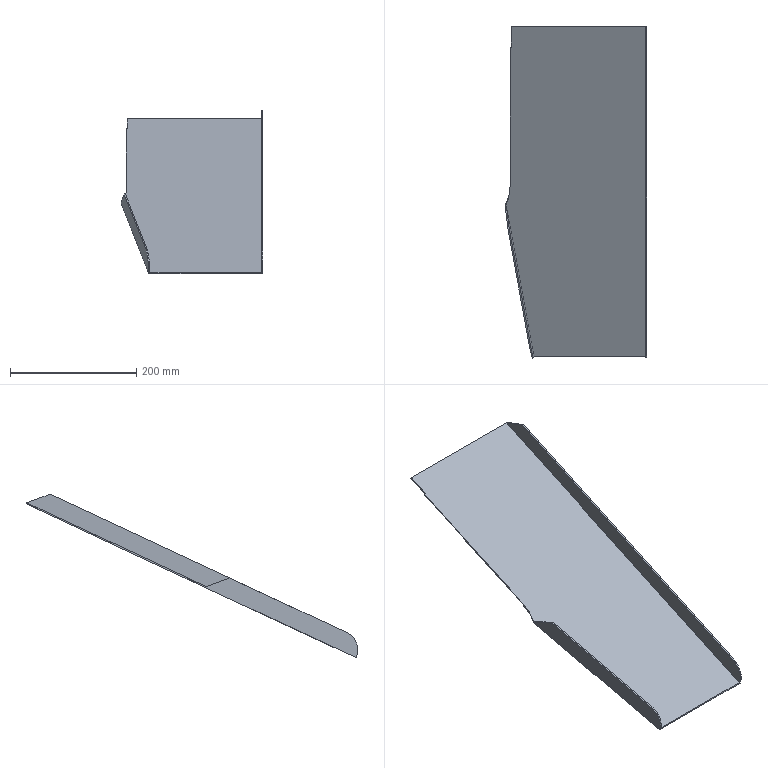Part | NX | features solid 2 | 1 solid | 19 faces | box 224.846 x 526.333 x 259.462 mm | volume 287368 mm3 | plane 15 | spline 2 | cylinder 2 | commonest cylinder face diameters 60 x2
STEP:
#1=CARTESIAN_POINT('',(1050.862,-840.,-297.376));
#2=VERTEX_POINT('',#1);
#3=CARTESIAN_POINT('',(1007.127,-602.381,-186.572));
#4=VERTEX_POINT('',#3);
#5=CARTESIAN_POINT('',(955.861,-323.845,-56.688));
#6=DIRECTION('',(-0.1645,0.894,0.4169));
#7=VECTOR('',#6,1000.);
#8=LINE('',#5,#7);
#9=EDGE_CURVE('',#2,#4,#8,.T.);
#10=ORIENTED_EDGE('',*,*,#9,.F.);
#11=CARTESIAN_POINT('',(1228.,-840.,-297.376));
#12=VERTEX_POINT('',#11);
#13=CARTESIAN_POINT('',(-1209.175,-840.,-297.376));
#14=DIRECTION('',(1.,0.,0.));
#15=VECTOR('',#14,1000.);
#16=LINE('',#13,#15);
#17=EDGE_CURVE('',#2,#12,#16,.T.);
#18=ORIENTED_EDGE('',*,*,#17,.T.);
#19=CARTESIAN_POINT('',(1228.,-317.358,-53.664));
#20=VERTEX_POINT('',#19);
#21=CARTESIAN_POINT('',(1228.,-651.161,-209.318));
#22=DIRECTION('',(0.,0.9063,0.4226));
#23=VECTOR('',#22,1000.);
#24=LINE('',#21,#23);
#25=EDGE_CURVE('',#12,#20,#24,.T.);
#26=ORIENTED_EDGE('',*,*,#25,.T.);
#27=CARTESIAN_POINT('',(1014.654,-317.358,-53.664));
#28=VERTEX_POINT('',#27);
#29=CARTESIAN_POINT('',(103.752,-317.358,-53.664));
#30=DIRECTION('',(-1.,0.,0.));
#31=VECTOR('',#30,1000.);
#32=LINE('',#29,#31);
#33=EDGE_CURVE('',#20,#28,#32,.T.);
#34=ORIENTED_EDGE('',*,*,#33,.T.);
#35=CARTESIAN_POINT('',(1014.619,-350.,-68.885));
#36=VERTEX_POINT('',#35);
#37=CARTESIAN_POINT('',(1014.654,-317.358,-53.664));
#38=CARTESIAN_POINT('',(1014.642,-328.239,-58.737));
#39=CARTESIAN_POINT('',(1014.63,-339.119,-63.811));
#40=CARTESIAN_POINT('',(1014.619,-350.,-68.885));
#41=B_SPLINE_CURVE_WITH_KNOTS('',3,(#37,#38,#39,#40),.UNSPECIFIED.,.F.,.F.,(4,4),(0.1137,0.1497),.UNSPECIFIED.);
#42=EDGE_CURVE('',#28,#36,#41,.T.);
#43=ORIENTED_EDGE('',*,*,#42,.T.);
#44=CARTESIAN_POINT('',(1013.163,-350.,-68.885));
#45=VERTEX_POINT('',#44);
#46=CARTESIAN_POINT('',(-1209.175,-350.,-68.885));
#47=DIRECTION('',(1.,0.,0.));
#48=VECTOR('',#47,1000.);
#49=LINE('',#46,#48);
#50=EDGE_CURVE('',#45,#36,#49,.T.);
#51=ORIENTED_EDGE('',*,*,#50,.F.);
#52=CARTESIAN_POINT('',(1005.271,-602.468,-186.613));
#53=VERTEX_POINT('',#52);
#54=CARTESIAN_POINT('',(1005.271,-602.468,-186.613));
#55=CARTESIAN_POINT('',(1007.853,-597.781,-184.427));
#56=CARTESIAN_POINT('',(1010.751,-589.874,-180.74));
#57=CARTESIAN_POINT('',(1012.652,-579.407,-175.859));
#58=CARTESIAN_POINT('',(1013.241,-571.511,-172.177));
#59=CARTESIAN_POINT('',(1013.239,-563.601,-168.488));
#60=CARTESIAN_POINT('',(1013.187,-553.051,-163.569));
#61=CARTESIAN_POINT('',(1013.19,-539.866,-157.421));
#62=CARTESIAN_POINT('',(1013.198,-524.044,-150.043));
#63=CARTESIAN_POINT('',(1013.2,-508.222,-142.665));
#64=CARTESIAN_POINT('',(1013.196,-492.4,-135.287));
#65=CARTESIAN_POINT('',(1013.191,-471.303,-125.45));
#66=CARTESIAN_POINT('',(1013.185,-444.933,-113.153));
#67=CARTESIAN_POINT('',(1013.175,-402.741,-93.478));
#68=CARTESIAN_POINT('',(1013.167,-371.096,-78.722));
#69=CARTESIAN_POINT('',(1013.163,-350.,-68.885));
#70=B_SPLINE_CURVE_WITH_KNOTS('',3,(#54,#55,#56,#57,#58,#59,#60,#61,#62,#63,#64,#65,#66,#67,#68,#69),.UNSPECIFIED.,.F.,.F.,(4,1,1,1,1,1,1,1,1,1,1,1,1,4),(0.2472,0.2642,0.2727,0.2812,0.2897,0.2982,0.3152,0.3322,0.3492,0.3662,0.3832,0.4172,0.4511,0.5191),.UNSPECIFIED.);
#71=EDGE_CURVE('',#53,#45,#70,.T.);
#72=ORIENTED_EDGE('',*,*,#71,.F.);
#73=CARTESIAN_POINT('',(1005.306,-602.656,-186.7));
#74=VERTEX_POINT('',#73);
#75=CARTESIAN_POINT('',(954.039,-324.12,-56.817));
#76=DIRECTION('',(-0.1645,0.894,0.4169));
#77=VECTOR('',#76,1000.);
#78=LINE('',#75,#77);
#79=EDGE_CURVE('',#74,#53,#78,.T.);
#80=ORIENTED_EDGE('',*,*,#79,.F.);
#81=CARTESIAN_POINT('',(1005.154,-602.679,-186.711));
#82=DIRECTION('',(0.9864,0.1491,0.06954));
#83=VECTOR('',#82,1000.);
#84=LINE('',#81,#83);
#85=EDGE_CURVE('',#74,#4,#84,.T.);
#86=ORIENTED_EDGE('',*,*,#85,.T.);
#87=EDGE_LOOP('',(#10,#18,#26,#34,#43,#51,#72,#80,#86));
#88=FACE_BOUND('',#87,.T.);
#89=CARTESIAN_POINT('',(-1209.175,-651.161,-209.318));
#90=DIRECTION('',(0.,-0.4226,0.9063));
#91=DIRECTION('',(1.,0.,0.));
#92=AXIS2_PLACEMENT_3D('',#89,#90,#91);
#93=PLANE('',#92);
#94=ADVANCED_FACE('',(#88),#93,.T.);
#95=CARTESIAN_POINT('',(1050.962,-840.,-298.783));
#96=VERTEX_POINT('',#95);
#97=CARTESIAN_POINT('',(1076.296,-840.,-658.146));
#98=DIRECTION('',(-0.07032,0.,0.9975));
#99=VECTOR('',#98,1000.);
#100=LINE('',#97,#99);
#101=EDGE_CURVE('',#96,#2,#100,.T.);
#102=ORIENTED_EDGE('',*,*,#101,.F.);
#103=CARTESIAN_POINT('',(1048.99,-840.,-299.582));
#104=VERTEX_POINT('',#103);
#105=CARTESIAN_POINT('',(866.662,-840.,-299.582));
#106=DIRECTION('',(0.,-1.,0.));
#107=DIRECTION('',(0.9975,0.,0.07032));
#108=AXIS2_PLACEMENT_3D('',#105,#106,#107);
#109=ELLIPSE('',#108,201.177,30.);
#110=EDGE_CURVE('',#104,#96,#109,.T.);
#111=ORIENTED_EDGE('',*,*,#110,.F.);
#112=CARTESIAN_POINT('',(1228.,-840.,-299.582));
#113=VERTEX_POINT('',#112);
#114=CARTESIAN_POINT('',(-1209.175,-840.,-299.582));
#115=DIRECTION('',(1.,0.,0.));
#116=VECTOR('',#115,1000.);
#117=LINE('',#114,#116);
#118=EDGE_CURVE('',#104,#113,#117,.T.);
#119=ORIENTED_EDGE('',*,*,#118,.T.);
#120=CARTESIAN_POINT('',(1228.,-840.,-660.));
#121=DIRECTION('',(0.,0.,1.));
#122=VECTOR('',#121,1000.);
#123=LINE('',#120,#122);
#124=EDGE_CURVE('',#113,#12,#123,.T.);
#125=ORIENTED_EDGE('',*,*,#124,.T.);
#126=ORIENTED_EDGE('',*,*,#17,.F.);
#127=EDGE_LOOP('',(#102,#111,#119,#125,#126));
#128=FACE_BOUND('',#127,.T.);
#129=CARTESIAN_POINT('',(1050.,-840.,-660.));
#130=DIRECTION('',(0.,-1.,0.));
#131=DIRECTION('',(0.,0.,-1.));
#132=AXIS2_PLACEMENT_3D('',#129,#130,#131);
#133=PLANE('',#132);
#134=ADVANCED_FACE('',(#128),#133,.T.);
#135=CARTESIAN_POINT('',(1005.154,-601.834,-188.524));
#136=VERTEX_POINT('',#135);
#137=CARTESIAN_POINT('',(953.888,-323.298,-58.64));
#138=DIRECTION('',(-0.1645,0.894,0.4169));
#139=VECTOR('',#138,1000.);
#140=LINE('',#137,#139);
#141=EDGE_CURVE('',#104,#136,#140,.T.);
#142=ORIENTED_EDGE('',*,*,#141,.T.);
#143=CARTESIAN_POINT('',(1013.163,-350.,-71.092));
#144=VERTEX_POINT('',#143);
#145=CARTESIAN_POINT('',(1005.154,-601.834,-188.524));
#146=CARTESIAN_POINT('',(1007.807,-597.071,-186.302));
#147=CARTESIAN_POINT('',(1010.57,-589.606,-182.822));
#148=CARTESIAN_POINT('',(1012.582,-579.13,-177.936));
#149=CARTESIAN_POINT('',(1013.224,-571.227,-174.251));
#150=CARTESIAN_POINT('',(1013.245,-563.328,-170.568));
#151=CARTESIAN_POINT('',(1013.186,-552.792,-165.655));
#152=CARTESIAN_POINT('',(1013.191,-539.624,-159.515));
#153=CARTESIAN_POINT('',(1013.197,-523.822,-152.146));
#154=CARTESIAN_POINT('',(1013.201,-502.753,-142.321));
#155=CARTESIAN_POINT('',(1013.192,-476.416,-130.04));
#156=CARTESIAN_POINT('',(1013.185,-444.812,-115.303));
#157=CARTESIAN_POINT('',(1013.175,-402.673,-95.654));
#158=CARTESIAN_POINT('',(1013.168,-371.069,-80.916));
#159=CARTESIAN_POINT('',(1013.163,-350.,-71.092));
#160=B_SPLINE_CURVE_WITH_KNOTS('',3,(#145,#146,#147,#148,#149,#150,#151,#152,#153,#154,#155,#156,#157,#158,#159),.UNSPECIFIED.,.F.,.F.,(4,1,1,1,1,1,1,1,1,1,1,1,4),(0.,0.0174,0.0261,0.0348,0.0435,0.0522,0.0696,0.087,0.1044,0.1392,0.174,0.2088,0.2784),.UNSPECIFIED.);
#161=EDGE_CURVE('',#136,#144,#160,.T.);
#162=ORIENTED_EDGE('',*,*,#161,.T.);
#163=CARTESIAN_POINT('',(1014.619,-350.,-71.092));
#164=VERTEX_POINT('',#163);
#165=CARTESIAN_POINT('',(-1209.175,-350.,-71.092));
#166=DIRECTION('',(1.,0.,0.));
#167=VECTOR('',#166,1000.);
#168=LINE('',#165,#167);
#169=EDGE_CURVE('',#144,#164,#168,.T.);
#170=ORIENTED_EDGE('',*,*,#169,.T.);
#171=CARTESIAN_POINT('',(1014.655,-316.513,-55.476));
#172=VERTEX_POINT('',#171);
#173=CARTESIAN_POINT('',(1014.655,-316.513,-55.476));
#174=CARTESIAN_POINT('',(1014.642,-327.675,-60.681));
#175=CARTESIAN_POINT('',(1014.631,-338.838,-65.886));
#176=CARTESIAN_POINT('',(1014.619,-350.,-71.092));
#177=B_SPLINE_CURVE_WITH_KNOTS('',3,(#173,#174,#175,#176),.UNSPECIFIED.,.F.,.F.,(4,4),(0.,0.03695),.UNSPECIFIED.);
#178=EDGE_CURVE('',#172,#164,#177,.T.);
#179=ORIENTED_EDGE('',*,*,#178,.F.);
#180=CARTESIAN_POINT('',(1230.,-316.513,-55.476));
#181=VERTEX_POINT('',#180);
#182=CARTESIAN_POINT('',(103.752,-316.513,-55.476));
#183=DIRECTION('',(-1.,0.,0.));
#184=VECTOR('',#183,1000.);
#185=LINE('',#182,#184);
#186=EDGE_CURVE('',#181,#172,#185,.T.);
#187=ORIENTED_EDGE('',*,*,#186,.F.);
#188=CARTESIAN_POINT('',(1230.,-840.,-299.582));
#189=VERTEX_POINT('',#188);
#190=CARTESIAN_POINT('',(1230.,-650.315,-211.131));
#191=DIRECTION('',(0.,-0.9063,-0.4226));
#192=VECTOR('',#191,1000.);
#193=LINE('',#190,#192);
#194=EDGE_CURVE('',#189,#181,#193,.F.);
#195=ORIENTED_EDGE('',*,*,#194,.F.);
#196=CARTESIAN_POINT('',(1230.,-840.,-299.582));
#197=DIRECTION('',(1.,0.,0.));
#198=VECTOR('',#197,1000.);
#199=LINE('',#196,#198);
#200=EDGE_CURVE('',#189,#113,#199,.F.);
#201=ORIENTED_EDGE('',*,*,#200,.T.);
#202=ORIENTED_EDGE('',*,*,#118,.F.);
#203=EDGE_LOOP('',(#142,#162,#170,#179,#187,#195,#201,#202));
#204=FACE_BOUND('',#203,.T.);
#205=CARTESIAN_POINT('',(-1209.175,-650.315,-211.131));
#206=DIRECTION('',(0.,-0.4226,0.9063));
#207=DIRECTION('',(1.,0.,0.));
#208=AXIS2_PLACEMENT_3D('',#205,#206,#207);
#209=PLANE('',#208);
#210=ADVANCED_FACE('',(#204),#209,.F.);
#211=ORIENTED_EDGE('',*,*,#186,.T.);
#212=CARTESIAN_POINT('',(1014.654,-317.358,-53.664));
#213=CARTESIAN_POINT('',(1014.654,-317.077,-54.268));
#214=CARTESIAN_POINT('',(1014.654,-316.795,-54.872));
#215=CARTESIAN_POINT('',(1014.655,-316.513,-55.476));
#216=B_SPLINE_CURVE_WITH_KNOTS('',3,(#212,#213,#214,#215),.UNSPECIFIED.,.F.,.F.,(4,4),(0.009777,0.01178),.UNSPECIFIED.);
#217=EDGE_CURVE('',#28,#172,#216,.T.);
#218=ORIENTED_EDGE('',*,*,#217,.F.);
#219=ORIENTED_EDGE('',*,*,#33,.F.);
#220=CARTESIAN_POINT('',(1230.,-317.358,-53.664));
#221=VERTEX_POINT('',#220);
#222=CARTESIAN_POINT('',(103.752,-317.358,-53.664));
#223=DIRECTION('',(-1.,0.,0.));
#224=VECTOR('',#223,1000.);
#225=LINE('',#222,#224);
#226=EDGE_CURVE('',#221,#20,#225,.T.);
#227=ORIENTED_EDGE('',*,*,#226,.F.);
#228=CARTESIAN_POINT('',(1230.,-317.358,-53.664));
#229=DIRECTION('',(0.,0.4226,-0.9063));
#230=VECTOR('',#229,1000.);
#231=LINE('',#228,#230);
#232=EDGE_CURVE('',#221,#181,#231,.T.);
#233=ORIENTED_EDGE('',*,*,#232,.T.);
#234=EDGE_LOOP('',(#211,#218,#219,#227,#233));
#235=FACE_BOUND('',#234,.T.);
#236=CARTESIAN_POINT('',(103.752,-317.358,-53.664));
#237=DIRECTION('',(0.,-0.9063,-0.4226));
#238=DIRECTION('',(0.,0.4226,-0.9063));
#239=AXIS2_PLACEMENT_3D('',#236,#237,#238);
#240=PLANE('',#239);
#241=ADVANCED_FACE('',(#235),#240,.F.);
#242=ORIENTED_EDGE('',*,*,#232,.F.);
#243=CARTESIAN_POINT('',(1230.,-354.568,-40.12));
#244=VERTEX_POINT('',#243);
#245=CARTESIAN_POINT('',(1230.,-699.826,85.543));
#246=DIRECTION('',(0.,-0.9397,0.342));
#247=VECTOR('',#246,1000.);
#248=LINE('',#245,#247);
#249=EDGE_CURVE('',#221,#244,#248,.T.);
#250=ORIENTED_EDGE('',*,*,#249,.T.);
#251=CARTESIAN_POINT('',(1230.,-825.489,-259.715));
#252=VERTEX_POINT('',#251);
#253=CARTESIAN_POINT('',(1230.,-852.679,-272.393));
#254=DIRECTION('',(0.,0.9063,0.4226));
#255=VECTOR('',#254,1000.);
#256=LINE('',#253,#255);
#257=EDGE_CURVE('',#252,#244,#256,.T.);
#258=ORIENTED_EDGE('',*,*,#257,.F.);
#259=CARTESIAN_POINT('',(1230.,-812.811,-286.904));
#260=DIRECTION('',(1.,0.,0.));
#261=DIRECTION('',(0.,0.,-1.));
#262=AXIS2_PLACEMENT_3D('',#259,#260,#261);
#263=CIRCLE('',#262,30.);
#264=EDGE_CURVE('',#252,#189,#263,.T.);
#265=ORIENTED_EDGE('',*,*,#264,.T.);
#266=ORIENTED_EDGE('',*,*,#194,.T.);
#267=EDGE_LOOP('',(#242,#250,#258,#265,#266));
#268=FACE_BOUND('',#267,.T.);
#269=CARTESIAN_POINT('',(1230.,-651.161,-209.318));
#270=DIRECTION('',(-1.,0.,0.));
#271=DIRECTION('',(0.,0.,1.));
#272=AXIS2_PLACEMENT_3D('',#269,#270,#271);
#273=PLANE('',#272);
#274=ADVANCED_FACE('',(#268),#273,.F.);
#275=CARTESIAN_POINT('',(1005.271,-602.468,-186.613));
#276=CARTESIAN_POINT('',(1005.232,-602.257,-187.25));
#277=CARTESIAN_POINT('',(1005.193,-602.046,-187.887));
#278=CARTESIAN_POINT('',(1005.154,-601.834,-188.524));
#279=B_SPLINE_CURVE_WITH_KNOTS('',3,(#275,#276,#277,#278),.UNSPECIFIED.,.F.,.F.,(4,4),(0.07169,0.0737),.UNSPECIFIED.);
#280=EDGE_CURVE('',#53,#136,#279,.T.);
#281=ORIENTED_EDGE('',*,*,#280,.T.);
#282=CARTESIAN_POINT('',(1005.154,-601.834,-188.524));
#283=DIRECTION('',(0.07546,-0.41,0.909));
#284=VECTOR('',#283,1000.);
#285=LINE('',#282,#284);
#286=EDGE_CURVE('',#136,#74,#285,.T.);
#287=ORIENTED_EDGE('',*,*,#286,.T.);
#288=ORIENTED_EDGE('',*,*,#79,.T.);
#289=EDGE_LOOP('',(#281,#287,#288));
#290=FACE_BOUND('',#289,.T.);
#291=CARTESIAN_POINT('',(1028.744,-730.,-248.288));
#292=DIRECTION('',(0.9835,0.181,0.));
#293=DIRECTION('',(-0.181,0.9835,0.));
#294=AXIS2_PLACEMENT_3D('',#291,#292,#293);
#295=PLANE('',#294);
#296=ADVANCED_FACE('',(#290),#295,.F.);
#297=CARTESIAN_POINT('',(1013.163,-350.,-71.092));
#298=CARTESIAN_POINT('',(1013.163,-350.,-70.356));
#299=CARTESIAN_POINT('',(1013.163,-350.,-69.62));
#300=CARTESIAN_POINT('',(1013.163,-350.,-68.885));
#301=B_SPLINE_CURVE_WITH_KNOTS('',3,(#297,#298,#299,#300),.UNSPECIFIED.,.F.,.F.,(4,4),(0.009839,0.01205),.UNSPECIFIED.);
#302=EDGE_CURVE('',#144,#45,#301,.T.);
#303=ORIENTED_EDGE('',*,*,#302,.F.);
#304=ORIENTED_EDGE('',*,*,#161,.F.);
#305=ORIENTED_EDGE('',*,*,#280,.F.);
#306=ORIENTED_EDGE('',*,*,#71,.T.);
#307=EDGE_LOOP('',(#303,#304,#305,#306));
#308=FACE_BOUND('',#307,.T.);
#309=CARTESIAN_POINT('',(1013.162,-348.314,-68.099));
#310=CARTESIAN_POINT('',(1013.162,-347.469,-69.911));
#311=CARTESIAN_POINT('',(1013.165,-360.164,-73.624));
#312=CARTESIAN_POINT('',(1013.165,-359.319,-75.437));
#313=CARTESIAN_POINT('',(1013.169,-377.939,-81.913));
#314=CARTESIAN_POINT('',(1013.169,-377.094,-83.726));
#315=CARTESIAN_POINT('',(1013.175,-401.639,-92.965));
#316=CARTESIAN_POINT('',(1013.175,-400.794,-94.777));
#317=CARTESIAN_POINT('',(1013.179,-419.414,-101.253));
#318=CARTESIAN_POINT('',(1013.179,-418.569,-103.066));
#319=CARTESIAN_POINT('',(1013.183,-437.189,-109.542));
#320=CARTESIAN_POINT('',(1013.183,-436.344,-111.354));
#321=CARTESIAN_POINT('',(1013.187,-454.964,-117.83));
#322=CARTESIAN_POINT('',(1013.187,-454.119,-119.643));
#323=CARTESIAN_POINT('',(1013.191,-469.778,-124.738));
#324=CARTESIAN_POINT('',(1013.191,-468.933,-126.551));
#325=CARTESIAN_POINT('',(1013.193,-481.625,-130.263));
#326=CARTESIAN_POINT('',(1013.193,-480.78,-132.075));
#327=CARTESIAN_POINT('',(1013.195,-489.038,-133.719));
#328=CARTESIAN_POINT('',(1013.195,-488.193,-135.532));
#329=CARTESIAN_POINT('',(1013.196,-494.95,-136.476));
#330=CARTESIAN_POINT('',(1013.196,-494.105,-138.289));
#331=CARTESIAN_POINT('',(1013.198,-500.93,-139.264));
#332=CARTESIAN_POINT('',(1013.198,-500.084,-141.077));
#333=CARTESIAN_POINT('',(1013.199,-506.472,-141.849));
#334=CARTESIAN_POINT('',(1013.199,-505.627,-143.662));
#335=CARTESIAN_POINT('',(1013.199,-511.465,-144.177));
#336=CARTESIAN_POINT('',(1013.199,-510.62,-145.99));
#337=CARTESIAN_POINT('',(1013.199,-514.954,-145.804));
#338=CARTESIAN_POINT('',(1013.199,-514.109,-147.617));
#339=CARTESIAN_POINT('',(1013.199,-518.182,-147.309));
#340=CARTESIAN_POINT('',(1013.199,-517.337,-149.122));
#341=CARTESIAN_POINT('',(1013.198,-520.655,-148.463));
#342=CARTESIAN_POINT('',(1013.198,-519.81,-150.275));
#343=CARTESIAN_POINT('',(1013.198,-522.504,-149.325));
#344=CARTESIAN_POINT('',(1013.198,-521.659,-151.137));
#345=CARTESIAN_POINT('',(1013.197,-523.825,-149.941));
#346=CARTESIAN_POINT('',(1013.197,-522.98,-151.753));
#347=CARTESIAN_POINT('',(1013.197,-524.873,-150.43));
#348=CARTESIAN_POINT('',(1013.197,-524.028,-152.242));
#349=CARTESIAN_POINT('',(1013.196,-525.575,-150.757));
#350=CARTESIAN_POINT('',(1013.196,-524.73,-152.57));
#351=CARTESIAN_POINT('',(1013.196,-525.974,-150.943));
#352=CARTESIAN_POINT('',(1013.196,-525.129,-152.755));
#353=CARTESIAN_POINT('',(1013.196,-526.253,-151.073));
#354=CARTESIAN_POINT('',(1013.196,-525.408,-152.886));
#355=CARTESIAN_POINT('',(1013.195,-526.948,-151.397));
#356=CARTESIAN_POINT('',(1013.195,-526.102,-153.209));
#357=CARTESIAN_POINT('',(1013.195,-527.718,-151.756));
#358=CARTESIAN_POINT('',(1013.195,-526.873,-153.569));
#359=CARTESIAN_POINT('',(1013.195,-528.718,-152.222));
#360=CARTESIAN_POINT('',(1013.195,-527.873,-154.035));
#361=CARTESIAN_POINT('',(1013.194,-529.873,-152.761));
#362=CARTESIAN_POINT('',(1013.194,-529.028,-154.574));
#363=CARTESIAN_POINT('',(1013.193,-531.391,-153.469));
#364=CARTESIAN_POINT('',(1013.193,-530.545,-155.281));
#365=CARTESIAN_POINT('',(1013.192,-533.227,-154.325));
#366=CARTESIAN_POINT('',(1013.192,-532.382,-156.138));
#367=CARTESIAN_POINT('',(1013.191,-536.045,-155.639));
#368=CARTESIAN_POINT('',(1013.191,-535.2,-157.452));
#369=CARTESIAN_POINT('',(1013.191,-539.337,-157.174));
#370=CARTESIAN_POINT('',(1013.191,-538.492,-158.987));
#371=CARTESIAN_POINT('',(1013.191,-542.922,-158.846));
#372=CARTESIAN_POINT('',(1013.191,-542.076,-160.658));
#373=CARTESIAN_POINT('',(1013.192,-546.139,-160.346));
#374=CARTESIAN_POINT('',(1013.192,-545.293,-162.158));
#375=CARTESIAN_POINT('',(1013.193,-548.513,-161.453));
#376=CARTESIAN_POINT('',(1013.193,-547.668,-163.265));
#377=CARTESIAN_POINT('',(1013.195,-550.23,-162.253));
#378=CARTESIAN_POINT('',(1013.195,-549.385,-164.066));
#379=CARTESIAN_POINT('',(1013.196,-551.422,-162.809));
#380=CARTESIAN_POINT('',(1013.196,-550.577,-164.622));
#381=CARTESIAN_POINT('',(1013.197,-552.35,-163.242));
#382=CARTESIAN_POINT('',(1013.197,-551.504,-165.055));
#383=CARTESIAN_POINT('',(1013.198,-553.022,-163.555));
#384=CARTESIAN_POINT('',(1013.198,-552.176,-165.368));
#385=CARTESIAN_POINT('',(1013.199,-553.477,-163.768));
#386=CARTESIAN_POINT('',(1013.199,-552.632,-165.58));
#387=CARTESIAN_POINT('',(1013.2,-553.705,-163.874));
#388=CARTESIAN_POINT('',(1013.2,-552.859,-165.686));
#389=CARTESIAN_POINT('',(1013.201,-554.382,-164.19));
#390=CARTESIAN_POINT('',(1013.201,-553.537,-166.002));
#391=CARTESIAN_POINT('',(1013.203,-555.372,-164.651));
#392=CARTESIAN_POINT('',(1013.203,-554.526,-166.464));
#393=CARTESIAN_POINT('',(1013.207,-556.843,-165.337));
#394=CARTESIAN_POINT('',(1013.207,-555.998,-167.15));
#395=CARTESIAN_POINT('',(1013.212,-558.233,-165.985));
#396=CARTESIAN_POINT('',(1013.212,-557.388,-167.798));
#397=CARTESIAN_POINT('',(1013.216,-559.317,-166.491));
#398=CARTESIAN_POINT('',(1013.216,-558.471,-168.303));
#399=CARTESIAN_POINT('',(1013.219,-559.994,-166.807));
#400=CARTESIAN_POINT('',(1013.219,-559.149,-168.619));
#401=CARTESIAN_POINT('',(1013.221,-560.435,-167.012));
#402=CARTESIAN_POINT('',(1013.221,-559.59,-168.825));
#403=CARTESIAN_POINT('',(1013.222,-560.727,-167.148));
#404=CARTESIAN_POINT('',(1013.222,-559.882,-168.961));
#405=CARTESIAN_POINT('',(1013.224,-561.19,-167.364));
#406=CARTESIAN_POINT('',(1013.224,-560.345,-169.177));
#407=CARTESIAN_POINT('',(1013.226,-561.69,-167.597));
#408=CARTESIAN_POINT('',(1013.226,-560.844,-169.41));
#409=CARTESIAN_POINT('',(1013.231,-562.884,-168.154));
#410=CARTESIAN_POINT('',(1013.231,-562.039,-169.967));
#411=CARTESIAN_POINT('',(1013.235,-564.449,-168.884));
#412=CARTESIAN_POINT('',(1013.235,-563.603,-170.696));
#413=CARTESIAN_POINT('',(1013.237,-565.828,-169.527));
#414=CARTESIAN_POINT('',(1013.237,-564.983,-171.34));
#415=CARTESIAN_POINT('',(1013.235,-566.723,-169.944));
#416=CARTESIAN_POINT('',(1013.235,-565.878,-171.757));
#417=CARTESIAN_POINT('',(1013.233,-567.178,-170.157));
#418=CARTESIAN_POINT('',(1013.233,-566.333,-171.969));
#419=CARTESIAN_POINT('',(1013.231,-567.489,-170.302));
#420=CARTESIAN_POINT('',(1013.231,-566.644,-172.114));
#421=CARTESIAN_POINT('',(1013.23,-567.601,-170.354));
#422=CARTESIAN_POINT('',(1013.23,-566.756,-172.167));
#423=CARTESIAN_POINT('',(1013.227,-567.909,-170.497));
#424=CARTESIAN_POINT('',(1013.227,-567.064,-172.31));
#425=CARTESIAN_POINT('',(1013.222,-568.336,-170.696));
#426=CARTESIAN_POINT('',(1013.222,-567.491,-172.509));
#427=CARTESIAN_POINT('',(1013.212,-568.985,-170.999));
#428=CARTESIAN_POINT('',(1013.212,-568.14,-172.812));
#429=CARTESIAN_POINT('',(1013.196,-569.789,-171.374));
#430=CARTESIAN_POINT('',(1013.196,-568.944,-173.187));
#431=CARTESIAN_POINT('',(1013.162,-571.041,-171.958));
#432=CARTESIAN_POINT('',(1013.162,-570.196,-173.771));
#433=CARTESIAN_POINT('',(1013.105,-572.539,-172.656));
#434=CARTESIAN_POINT('',(1013.105,-571.694,-174.469));
#435=CARTESIAN_POINT('',(1013.025,-573.995,-173.335));
#436=CARTESIAN_POINT('',(1013.025,-573.15,-175.148));
#437=CARTESIAN_POINT('',(1012.954,-575.038,-173.822));
#438=CARTESIAN_POINT('',(1012.954,-574.193,-175.634));
#439=CARTESIAN_POINT('',(1012.85,-576.362,-174.439));
#440=CARTESIAN_POINT('',(1012.85,-575.516,-176.252));
#441=CARTESIAN_POINT('',(1012.637,-578.533,-175.452));
#442=CARTESIAN_POINT('',(1012.637,-577.688,-177.264));
#443=CARTESIAN_POINT('',(1012.307,-581.001,-176.603));
#444=CARTESIAN_POINT('',(1012.307,-580.156,-178.415));
#445=CARTESIAN_POINT('',(1011.874,-583.508,-177.772));
#446=CARTESIAN_POINT('',(1011.874,-582.663,-179.584));
#447=CARTESIAN_POINT('',(1011.349,-586.133,-178.996));
#448=CARTESIAN_POINT('',(1011.349,-585.288,-180.808));
#449=CARTESIAN_POINT('',(1010.577,-589.296,-180.47));
#450=CARTESIAN_POINT('',(1010.577,-588.45,-182.283));
#451=CARTESIAN_POINT('',(1009.631,-592.391,-181.913));
#452=CARTESIAN_POINT('',(1009.631,-591.546,-183.726));
#453=CARTESIAN_POINT('',(1008.775,-594.801,-183.037));
#454=CARTESIAN_POINT('',(1008.775,-593.956,-184.85));
#455=CARTESIAN_POINT('',(1008.19,-596.299,-183.736));
#456=CARTESIAN_POINT('',(1008.19,-595.454,-185.549));
#457=CARTESIAN_POINT('',(1007.711,-597.449,-184.272));
#458=CARTESIAN_POINT('',(1007.711,-596.604,-186.085));
#459=CARTESIAN_POINT('',(1007.16,-598.714,-184.862));
#460=CARTESIAN_POINT('',(1007.16,-597.868,-186.674));
#461=CARTESIAN_POINT('',(1006.081,-601.013,-185.934));
#462=CARTESIAN_POINT('',(1006.081,-600.167,-187.746));
#463=CARTESIAN_POINT('',(1005.074,-602.861,-186.796));
#464=CARTESIAN_POINT('',(1005.074,-602.016,-188.609));
#465=CARTESIAN_POINT('',(1004.352,-604.068,-187.359));
#466=CARTESIAN_POINT('',(1004.352,-603.223,-189.171));
#467=B_SPLINE_SURFACE_WITH_KNOTS('',3,1,((#309,#310),(#311,#312),(#313,#314),(#315,#316),(#317,#318),(#319,#320),(#321,#322),(#323,#324),(#325,#326),(#327,#328),(#329,#330),(#331,#332),(#333,#334),(#335,#336),(#337,#338),(#339,#340),(#341,#342),(#343,#344),(#345,#346),(#347,#348),(#349,#350),(#351,#352),(#353,#354),(#355,#356),(#357,#358),(#359,#360),(#361,#362),(#363,#364),(#365,#366),(#367,#368),(#369,#370),(#371,#372),(#373,#374),(#375,#376),(#377,#378),(#379,#380),(#381,#382),(#383,#384),(#385,#386),(#387,#388),(#389,#390),(#391,#392),(#393,#394),(#395,#396),(#397,#398),(#399,#400),(#401,#402),(#403,#404),(#405,#406),(#407,#408),(#409,#410),(#411,#412),(#413,#414),(#415,#416),(#417,#418),(#419,#420),(#421,#422),(#423,#424),(#425,#426),(#427,#428),(#429,#430),(#431,#432),(#433,#434),(#435,#436),(#437,#438),(#439,#440),(#441,#442),(#443,#444),(#445,#446),(#447,#448),(#449,#450),(#451,#452),(#453,#454),(#455,#456),(#457,#458),(#459,#460),(#461,#462),(#463,#464),(#465,#466)),.SURF_OF_LINEAR_EXTRUSION.,.F.,.F.,.F.,(4,1,1,1,1,1,1,1,1,1,1,1,1,1,1,1,1,1,1,1,1,1,1,1,1,1,1,1,1,1,1,1,1,1,1,1,1,1,1,1,1,1,1,1,1,1,1,1,1,1,1,1,1,1,1,1,1,1,1,1,1,1,1,1,1,1,1,1,1,1,1,1,1,1,1,1,4),(2,2),(-1.037,-0.7918,-0.6692,-0.5465,-0.4239,-0.3012,-0.1786,-0.1172,-0.05592,-0.02525,0.005411,0.06674,0.0974,0.1281,0.1587,0.1894,0.2047,0.2201,0.2354,0.2431,0.2469,0.2507,0.2546,0.2584,0.2661,0.2737,0.2814,0.2967,0.312,0.3427,0.3734,0.404,0.4347,0.45,0.4654,0.4807,0.4884,0.496,0.4999,0.5037,0.5114,0.5267,0.542,0.5497,0.5574,0.5612,0.5631,0.565,0.5689,0.5727,0.588,0.6034,0.611,0.6187,0.6225,0.6244,0.6264,0.6302,0.634,0.6417,0.6493,0.6647,0.68,0.6877,0.6953,0.7107,0.7413,0.7567,0.772,0.8027,0.8333,0.8487,0.864,0.8717,0.8793,0.8947,0.9253),(0.,1.),.UNSPECIFIED.);
#468=ADVANCED_FACE('',(#308),#467,.F.);
#469=ORIENTED_EDGE('',*,*,#217,.T.);
#470=ORIENTED_EDGE('',*,*,#178,.T.);
#471=CARTESIAN_POINT('',(1014.619,-350.,-69.988));
#472=DIRECTION('',(0.,0.,-1.));
#473=VECTOR('',#472,1000.);
#474=LINE('',#471,#473);
#475=EDGE_CURVE('',#164,#36,#474,.F.);
#476=ORIENTED_EDGE('',*,*,#475,.T.);
#477=ORIENTED_EDGE('',*,*,#42,.F.);
#478=EDGE_LOOP('',(#469,#470,#476,#477));
#479=FACE_BOUND('',#478,.T.);
#480=CARTESIAN_POINT('',(1014.619,-350.,-59.72));
#481=CARTESIAN_POINT('',(1014.619,-350.,-71.159));
#482=CARTESIAN_POINT('',(1014.631,-338.786,-57.53));
#483=CARTESIAN_POINT('',(1014.631,-338.786,-68.969));
#484=CARTESIAN_POINT('',(1014.643,-327.547,-55.48));
#485=CARTESIAN_POINT('',(1014.643,-327.547,-66.92));
#486=CARTESIAN_POINT('',(1014.655,-316.312,-53.402));
#487=CARTESIAN_POINT('',(1014.655,-316.312,-64.842));
#488=B_SPLINE_SURFACE_WITH_KNOTS('',3,1,((#480,#481),(#482,#483),(#484,#485),(#486,#487)),.SURF_OF_LINEAR_EXTRUSION.,.F.,.F.,.F.,(4,4),(2,2),(0.02311,0.1805),(0.,1.),.PIECEWISE_BEZIER_KNOTS.);
#489=ADVANCED_FACE('',(#479),#488,.T.);
#490=ORIENTED_EDGE('',*,*,#50,.T.);
#491=ORIENTED_EDGE('',*,*,#475,.F.);
#492=ORIENTED_EDGE('',*,*,#169,.F.);
#493=ORIENTED_EDGE('',*,*,#302,.T.);
#494=EDGE_LOOP('',(#490,#491,#492,#493));
#495=FACE_BOUND('',#494,.T.);
#496=CARTESIAN_POINT('',(802.881,-350.,-63.258));
#497=DIRECTION('',(0.,-1.,0.));
#498=DIRECTION('',(0.,0.,-1.));
#499=AXIS2_PLACEMENT_3D('',#496,#497,#498);
#500=PLANE('',#499);
#501=ADVANCED_FACE('',(#495),#500,.F.);
#502=ORIENTED_EDGE('',*,*,#257,.T.);
#503=CARTESIAN_POINT('',(1228.,-354.568,-40.12));
#504=VERTEX_POINT('',#503);
#505=CARTESIAN_POINT('',(1230.,-354.568,-40.12));
#506=DIRECTION('',(-1.,0.,0.));
#507=VECTOR('',#506,1000.);
#508=LINE('',#505,#507);
#509=EDGE_CURVE('',#244,#504,#508,.T.);
#510=ORIENTED_EDGE('',*,*,#509,.T.);
#511=CARTESIAN_POINT('',(1228.,-825.489,-259.715));
#512=VERTEX_POINT('',#511);
#513=CARTESIAN_POINT('',(1228.,-852.679,-272.393));
#514=DIRECTION('',(0.,0.9063,0.4226));
#515=VECTOR('',#514,1000.);
#516=LINE('',#513,#515);
#517=EDGE_CURVE('',#512,#504,#516,.T.);
#518=ORIENTED_EDGE('',*,*,#517,.F.);
#519=CARTESIAN_POINT('',(1230.,-825.489,-259.715));
#520=DIRECTION('',(-1.,0.,0.));
#521=VECTOR('',#520,1000.);
#522=LINE('',#519,#521);
#523=EDGE_CURVE('',#512,#252,#522,.F.);
#524=ORIENTED_EDGE('',*,*,#523,.T.);
#525=EDGE_LOOP('',(#502,#510,#518,#524));
#526=FACE_BOUND('',#525,.T.);
#527=CARTESIAN_POINT('',(1230.,-852.679,-272.393));
#528=DIRECTION('',(0.,0.4226,-0.9063));
#529=DIRECTION('',(0.,0.9063,0.4226));
#530=AXIS2_PLACEMENT_3D('',#527,#528,#529);
#531=PLANE('',#530);
#532=ADVANCED_FACE('',(#526),#531,.F.);
#533=ORIENTED_EDGE('',*,*,#25,.F.);
#534=ORIENTED_EDGE('',*,*,#124,.F.);
#535=CARTESIAN_POINT('',(1228.,-812.811,-286.904));
#536=DIRECTION('',(1.,0.,0.));
#537=DIRECTION('',(0.,0.,-1.));
#538=AXIS2_PLACEMENT_3D('',#535,#536,#537);
#539=CIRCLE('',#538,30.);
#540=EDGE_CURVE('',#113,#512,#539,.F.);
#541=ORIENTED_EDGE('',*,*,#540,.T.);
#542=ORIENTED_EDGE('',*,*,#517,.T.);
#543=CARTESIAN_POINT('',(1228.,-354.568,-40.12));
#544=DIRECTION('',(0.,0.9397,-0.342));
#545=VECTOR('',#544,1000.);
#546=LINE('',#543,#545);
#547=EDGE_CURVE('',#504,#20,#546,.T.);
#548=ORIENTED_EDGE('',*,*,#547,.T.);
#549=EDGE_LOOP('',(#533,#534,#541,#542,#548));
#550=FACE_BOUND('',#549,.T.);
#551=CARTESIAN_POINT('',(1228.,-840.,-299.582));
#552=DIRECTION('',(1.,0.,0.));
#553=DIRECTION('',(0.,0.,-1.));
#554=AXIS2_PLACEMENT_3D('',#551,#552,#553);
#555=PLANE('',#554);
#556=ADVANCED_FACE('',(#550),#555,.F.);
#557=ORIENTED_EDGE('',*,*,#264,.F.);
#558=ORIENTED_EDGE('',*,*,#523,.F.);
#559=ORIENTED_EDGE('',*,*,#540,.F.);
#560=ORIENTED_EDGE('',*,*,#200,.F.);
#561=EDGE_LOOP('',(#557,#558,#559,#560));
#562=FACE_BOUND('',#561,.T.);
#563=CARTESIAN_POINT('',(1230.,-812.811,-286.904));
#564=DIRECTION('',(-1.,0.,0.));
#565=DIRECTION('',(0.,0.,1.));
#566=AXIS2_PLACEMENT_3D('',#563,#564,#565);
#567=CYLINDRICAL_SURFACE('',#566,30.);
#568=ADVANCED_FACE('',(#562),#567,.T.);
#569=ORIENTED_EDGE('',*,*,#249,.F.);
#570=ORIENTED_EDGE('',*,*,#226,.T.);
#571=ORIENTED_EDGE('',*,*,#547,.F.);
#572=ORIENTED_EDGE('',*,*,#509,.F.);
#573=EDGE_LOOP('',(#569,#570,#571,#572));
#574=FACE_BOUND('',#573,.T.);
#575=CARTESIAN_POINT('',(1230.,-354.568,-40.12));
#576=DIRECTION('',(0.,0.342,0.9397));
#577=DIRECTION('',(0.,-0.9397,0.342));
#578=AXIS2_PLACEMENT_3D('',#575,#576,#577);
#579=PLANE('',#578);
#580=ADVANCED_FACE('',(#574),#579,.T.);
#581=ORIENTED_EDGE('',*,*,#286,.F.);
#582=CARTESIAN_POINT('',(1005.154,-602.679,-186.711));
#583=VERTEX_POINT('',#582);
#584=CARTESIAN_POINT('',(1005.154,-601.834,-188.524));
#585=DIRECTION('',(0.,-0.4226,0.9063));
#586=VECTOR('',#585,1000.);
#587=LINE('',#584,#586);
#588=EDGE_CURVE('',#136,#583,#587,.T.);
#589=ORIENTED_EDGE('',*,*,#588,.T.);
#590=CARTESIAN_POINT('',(1005.154,-602.679,-186.711));
#591=DIRECTION('',(0.9864,0.1491,0.06954));
#592=VECTOR('',#591,1000.);
#593=LINE('',#590,#592);
#594=EDGE_CURVE('',#583,#74,#593,.T.);
#595=ORIENTED_EDGE('',*,*,#594,.T.);
#596=EDGE_LOOP('',(#581,#589,#595));
#597=FACE_BOUND('',#596,.T.);
#598=CARTESIAN_POINT('',(1005.154,-601.834,-188.524));
#599=DIRECTION('',(-0.1645,0.894,0.4169));
#600=DIRECTION('',(0.,-0.4226,0.9063));
#601=AXIS2_PLACEMENT_3D('',#598,#599,#600);
#602=PLANE('',#601);
#603=ADVANCED_FACE('',(#597),#602,.T.);
#604=CARTESIAN_POINT('',(1046.027,-825.562,-259.748));
#605=VERTEX_POINT('',#604);
#606=CARTESIAN_POINT('',(1011.734,-639.245,-172.867));
#607=VERTEX_POINT('',#606);
#608=CARTESIAN_POINT('',(1050.963,-852.38,-272.254));
#609=DIRECTION('',(0.1645,-0.894,-0.4169));
#610=VECTOR('',#609,1000.);
#611=LINE('',#608,#610);
#612=EDGE_CURVE('',#605,#607,#611,.F.);
#613=ORIENTED_EDGE('',*,*,#612,.T.);
#614=CARTESIAN_POINT('',(1009.761,-639.543,-173.006));
#615=VERTEX_POINT('',#614);
#616=CARTESIAN_POINT('',(1009.761,-639.543,-173.006));
#617=DIRECTION('',(0.9864,0.1491,0.06954));
#618=VECTOR('',#617,1000.);
#619=LINE('',#616,#618);
#620=EDGE_CURVE('',#607,#615,#619,.F.);
#621=ORIENTED_EDGE('',*,*,#620,.T.);
#622=CARTESIAN_POINT('',(1044.054,-825.86,-259.887));
#623=VERTEX_POINT('',#622);
#624=CARTESIAN_POINT('',(1048.99,-852.679,-272.393));
#625=DIRECTION('',(0.1645,-0.894,-0.4169));
#626=VECTOR('',#625,1000.);
#627=LINE('',#624,#626);
#628=EDGE_CURVE('',#623,#615,#627,.F.);
#629=ORIENTED_EDGE('',*,*,#628,.F.);
#630=CARTESIAN_POINT('',(1044.054,-825.86,-259.887));
#631=DIRECTION('',(-0.9864,-0.1491,-0.06954));
#632=VECTOR('',#631,1000.);
#633=LINE('',#630,#632);
#634=EDGE_CURVE('',#623,#605,#633,.F.);
#635=ORIENTED_EDGE('',*,*,#634,.T.);
#636=EDGE_LOOP('',(#613,#621,#629,#635));
#637=FACE_BOUND('',#636,.T.);
#638=CARTESIAN_POINT('',(1048.99,-852.679,-272.393));
#639=DIRECTION('',(0.,0.4226,-0.9063));
#640=DIRECTION('',(-0.1645,0.894,0.4169));
#641=AXIS2_PLACEMENT_3D('',#638,#639,#640);
#642=PLANE('',#641);
#643=ADVANCED_FACE('',(#637),#642,.F.);
#644=ORIENTED_EDGE('',*,*,#101,.T.);
#645=ORIENTED_EDGE('',*,*,#9,.T.);
#646=CARTESIAN_POINT('',(1028.88,-776.444,-121.862));
#647=DIRECTION('',(0.1163,-0.931,0.3461));
#648=VECTOR('',#647,1000.);
#649=LINE('',#646,#648);
#650=EDGE_CURVE('',#4,#607,#649,.T.);
#651=ORIENTED_EDGE('',*,*,#650,.T.);
#652=ORIENTED_EDGE('',*,*,#612,.F.);
#653=CARTESIAN_POINT('',(1046.027,-812.883,-286.937));
#654=DIRECTION('',(0.9864,0.1491,0.06954));
#655=DIRECTION('',(-0.1495,0.9888,0.));
#656=AXIS2_PLACEMENT_3D('',#653,#654,#655);
#657=CIRCLE('',#656,30.);
#658=EDGE_CURVE('',#605,#96,#657,.T.);
#659=ORIENTED_EDGE('',*,*,#658,.T.);
#660=EDGE_LOOP('',(#644,#645,#651,#652,#659));
#661=FACE_BOUND('',#660,.T.);
#662=CARTESIAN_POINT('',(1050.963,-839.702,-299.443));
#663=DIRECTION('',(0.9864,0.1491,0.06954));
#664=DIRECTION('',(-0.1495,0.9888,0.));
#665=AXIS2_PLACEMENT_3D('',#662,#663,#664);
#666=PLANE('',#665);
#667=ADVANCED_FACE('',(#661),#666,.T.);
#668=ORIENTED_EDGE('',*,*,#628,.T.);
#669=CARTESIAN_POINT('',(1005.154,-602.679,-186.711));
#670=DIRECTION('',(-0.1163,0.931,-0.3461));
#671=VECTOR('',#670,1000.);
#672=LINE('',#669,#671);
#673=EDGE_CURVE('',#615,#583,#672,.T.);
#674=ORIENTED_EDGE('',*,*,#673,.T.);
#675=ORIENTED_EDGE('',*,*,#588,.F.);
#676=ORIENTED_EDGE('',*,*,#141,.F.);
#677=CARTESIAN_POINT('',(1044.054,-813.181,-287.077));
#678=DIRECTION('',(0.9864,0.1491,0.06954));
#679=DIRECTION('',(-0.1495,0.9888,0.));
#680=AXIS2_PLACEMENT_3D('',#677,#678,#679);
#681=CIRCLE('',#680,30.);
#682=EDGE_CURVE('',#104,#623,#681,.F.);
#683=ORIENTED_EDGE('',*,*,#682,.T.);
#684=EDGE_LOOP('',(#668,#674,#675,#676,#683));
#685=FACE_BOUND('',#684,.T.);
#686=CARTESIAN_POINT('',(1048.99,-840.,-299.582));
#687=DIRECTION('',(0.9864,0.1491,0.06954));
#688=DIRECTION('',(-0.1495,0.9888,0.));
#689=AXIS2_PLACEMENT_3D('',#686,#687,#688);
#690=PLANE('',#689);
#691=ADVANCED_FACE('',(#685),#690,.F.);
#692=ORIENTED_EDGE('',*,*,#682,.F.);
#693=ORIENTED_EDGE('',*,*,#110,.T.);
#694=ORIENTED_EDGE('',*,*,#658,.F.);
#695=ORIENTED_EDGE('',*,*,#634,.F.);
#696=EDGE_LOOP('',(#692,#693,#694,#695));
#697=FACE_BOUND('',#696,.T.);
#698=CARTESIAN_POINT('',(1044.054,-813.181,-287.077));
#699=DIRECTION('',(0.9864,0.1491,0.06954));
#700=DIRECTION('',(-0.1495,0.9888,0.));
#701=AXIS2_PLACEMENT_3D('',#698,#699,#700);
#702=CYLINDRICAL_SURFACE('',#701,30.);
#703=ADVANCED_FACE('',(#697),#702,.T.);
#704=ORIENTED_EDGE('',*,*,#673,.F.);
#705=ORIENTED_EDGE('',*,*,#620,.F.);
#706=ORIENTED_EDGE('',*,*,#650,.F.);
#707=ORIENTED_EDGE('',*,*,#85,.F.);
#708=ORIENTED_EDGE('',*,*,#594,.F.);
#709=EDGE_LOOP('',(#704,#705,#706,#707,#708));
#710=FACE_BOUND('',#709,.T.);
#711=CARTESIAN_POINT('',(1005.154,-602.679,-186.711));
#712=DIRECTION('',(-0.1163,0.3333,0.9356));
#713=DIRECTION('',(0.,-0.942,0.3356));
#714=AXIS2_PLACEMENT_3D('',#711,#712,#713);
#715=PLANE('',#714);
#716=ADVANCED_FACE('',(#710),#715,.T.);
#717=CLOSED_SHELL('',(#94,#134,#210,#241,#274,#296,#468,#489,#501,#532,#556,#568,#580,#603,#643,#667,#691,#703,#716));
#718=MANIFOLD_SOLID_BREP('',#717);
#719=(LENGTH_UNIT()NAMED_UNIT(*)SI_UNIT(.MILLI.,.METRE.));
#720=UNCERTAINTY_MEASURE_WITH_UNIT(LENGTH_MEASURE(0.0508),#719,'','');
#721=(NAMED_UNIT(*)PLANE_ANGLE_UNIT()SI_UNIT($,.RADIAN.));
#722=(NAMED_UNIT(*)SI_UNIT($,.STERADIAN.)SOLID_ANGLE_UNIT());
#723=(GEOMETRIC_REPRESENTATION_CONTEXT(3)GLOBAL_UNCERTAINTY_ASSIGNED_CONTEXT((#720))GLOBAL_UNIT_ASSIGNED_CONTEXT((#719,#721,#722))REPRESENTATION_CONTEXT('',''));
#724=ADVANCED_BREP_SHAPE_REPRESENTATION('',(#718),#723);